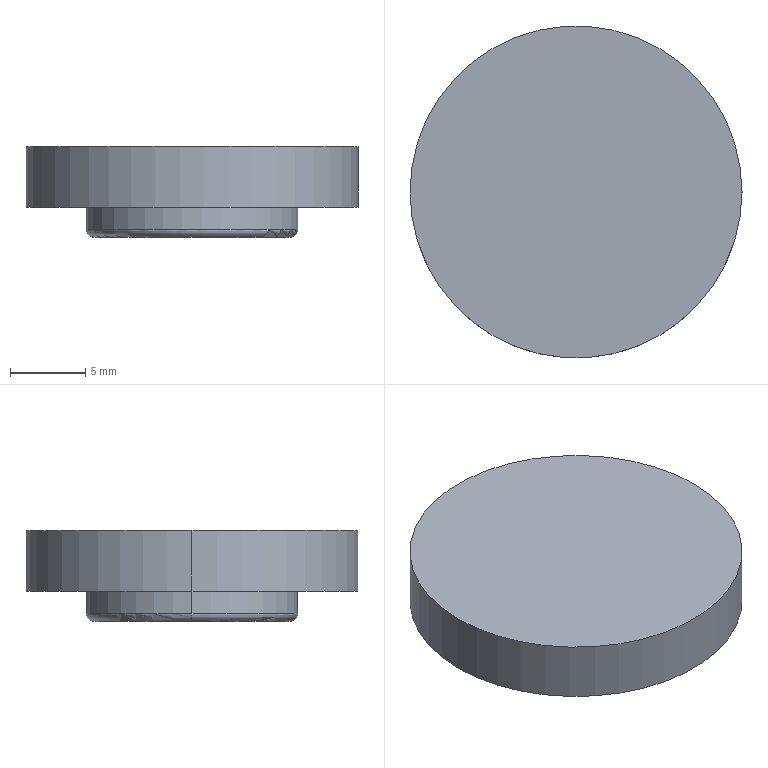Part | 1 solid | 9 faces | box 22 x 22 x 6 mm | volume 1826 mm3 | cylinder 4 | plane 3 | torus 2 | commonest cylinder face diameters 14 x2 22 x2
STEP:
#1=CARTESIAN_POINT('',(-6.5,0.,0.));
#2=VERTEX_POINT('',#1);
#3=CARTESIAN_POINT('',(6.5,0.,0.));
#4=VERTEX_POINT('',#3);
#5=CARTESIAN_POINT('',(0.,0.,0.));
#6=DIRECTION('',(0.,0.,-1.));
#7=DIRECTION('',(1.,0.,0.));
#8=AXIS2_PLACEMENT_3D('',#5,#6,#7);
#9=CIRCLE('',#8,6.5);
#10=EDGE_CURVE('',#2,#4,#9,.T.);
#11=ORIENTED_EDGE('',*,*,#10,.F.);
#12=CARTESIAN_POINT('',(-7.,0.,0.5));
#13=VERTEX_POINT('',#12);
#14=CARTESIAN_POINT('',(-6.5,0.,0.5));
#15=DIRECTION('',(0.,1.,0.));
#16=DIRECTION('',(-1.,0.,0.));
#17=AXIS2_PLACEMENT_3D('',#14,#15,#16);
#18=CIRCLE('',#17,0.5);
#19=EDGE_CURVE('',#2,#13,#18,.T.);
#20=ORIENTED_EDGE('',*,*,#19,.T.);
#21=CARTESIAN_POINT('',(7.,0.,0.5));
#22=VERTEX_POINT('',#21);
#23=CARTESIAN_POINT('',(0.,0.,0.5));
#24=DIRECTION('',(0.,0.,1.));
#25=DIRECTION('',(1.,0.,0.));
#26=AXIS2_PLACEMENT_3D('',#23,#24,#25);
#27=CIRCLE('',#26,7.);
#28=EDGE_CURVE('',#22,#13,#27,.T.);
#29=ORIENTED_EDGE('',*,*,#28,.F.);
#30=CARTESIAN_POINT('',(6.5,0.,0.5));
#31=DIRECTION('',(0.,-1.,0.));
#32=DIRECTION('',(0.,0.,-1.));
#33=AXIS2_PLACEMENT_3D('',#30,#31,#32);
#34=CIRCLE('',#33,0.5);
#35=EDGE_CURVE('',#4,#22,#34,.T.);
#36=ORIENTED_EDGE('',*,*,#35,.F.);
#37=EDGE_LOOP('',(#11,#20,#29,#36));
#38=FACE_OUTER_BOUND('',#37,.T.);
#39=CARTESIAN_POINT('',(0.,0.,0.5));
#40=DIRECTION('',(0.,0.,1.));
#41=DIRECTION('',(1.,0.,0.));
#42=AXIS2_PLACEMENT_3D('',#39,#40,#41);
#43=TOROIDAL_SURFACE('',#42,6.5,0.5);
#44=ADVANCED_FACE('',(#38),#43,.T.);
#45=CARTESIAN_POINT('',(11.,0.,6.));
#46=VERTEX_POINT('',#45);
#47=CARTESIAN_POINT('',(-11.,0.,6.));
#48=VERTEX_POINT('',#47);
#49=CARTESIAN_POINT('',(0.,0.,6.));
#50=DIRECTION('',(0.,0.,1.));
#51=DIRECTION('',(1.,0.,0.));
#52=AXIS2_PLACEMENT_3D('',#49,#50,#51);
#53=CIRCLE('',#52,11.);
#54=EDGE_CURVE('',#46,#48,#53,.T.);
#55=ORIENTED_EDGE('',*,*,#54,.F.);
#56=CARTESIAN_POINT('',(11.,0.,2.));
#57=VERTEX_POINT('',#56);
#58=CARTESIAN_POINT('',(11.,0.,6.));
#59=DIRECTION('',(0.,0.,-1.));
#60=VECTOR('',#59,1000.);
#61=LINE('',#58,#60);
#62=EDGE_CURVE('',#46,#57,#61,.T.);
#63=ORIENTED_EDGE('',*,*,#62,.T.);
#64=CARTESIAN_POINT('',(-11.,0.,2.));
#65=VERTEX_POINT('',#64);
#66=CARTESIAN_POINT('',(0.,0.,2.));
#67=DIRECTION('',(0.,0.,1.));
#68=DIRECTION('',(1.,0.,0.));
#69=AXIS2_PLACEMENT_3D('',#66,#67,#68);
#70=CIRCLE('',#69,11.);
#71=EDGE_CURVE('',#57,#65,#70,.T.);
#72=ORIENTED_EDGE('',*,*,#71,.T.);
#73=CARTESIAN_POINT('',(-11.,0.,6.));
#74=DIRECTION('',(0.,0.,-1.));
#75=VECTOR('',#74,1000.);
#76=LINE('',#73,#75);
#77=EDGE_CURVE('',#48,#65,#76,.T.);
#78=ORIENTED_EDGE('',*,*,#77,.F.);
#79=EDGE_LOOP('',(#55,#63,#72,#78));
#80=FACE_OUTER_BOUND('',#79,.T.);
#81=CARTESIAN_POINT('',(0.,0.,6.));
#82=DIRECTION('',(0.,0.,-1.));
#83=DIRECTION('',(-1.,0.,0.));
#84=AXIS2_PLACEMENT_3D('',#81,#82,#83);
#85=CYLINDRICAL_SURFACE('',#84,11.);
#86=ADVANCED_FACE('',(#80),#85,.T.);
#87=CARTESIAN_POINT('',(7.,0.,2.));
#88=VERTEX_POINT('',#87);
#89=CARTESIAN_POINT('',(-7.,0.,2.));
#90=VERTEX_POINT('',#89);
#91=CARTESIAN_POINT('',(0.,0.,2.));
#92=DIRECTION('',(0.,0.,1.));
#93=DIRECTION('',(1.,0.,0.));
#94=AXIS2_PLACEMENT_3D('',#91,#92,#93);
#95=CIRCLE('',#94,7.);
#96=EDGE_CURVE('',#88,#90,#95,.T.);
#97=ORIENTED_EDGE('',*,*,#96,.F.);
#98=CARTESIAN_POINT('',(7.,0.,2.));
#99=DIRECTION('',(0.,0.,-1.));
#100=VECTOR('',#99,1000.);
#101=LINE('',#98,#100);
#102=EDGE_CURVE('',#88,#22,#101,.T.);
#103=ORIENTED_EDGE('',*,*,#102,.T.);
#104=ORIENTED_EDGE('',*,*,#28,.T.);
#105=CARTESIAN_POINT('',(-7.,0.,2.));
#106=DIRECTION('',(0.,0.,-1.));
#107=VECTOR('',#106,1000.);
#108=LINE('',#105,#107);
#109=EDGE_CURVE('',#90,#13,#108,.T.);
#110=ORIENTED_EDGE('',*,*,#109,.F.);
#111=EDGE_LOOP('',(#97,#103,#104,#110));
#112=FACE_OUTER_BOUND('',#111,.T.);
#113=CARTESIAN_POINT('',(0.,0.,2.));
#114=DIRECTION('',(0.,0.,-1.));
#115=DIRECTION('',(-1.,0.,0.));
#116=AXIS2_PLACEMENT_3D('',#113,#114,#115);
#117=CYLINDRICAL_SURFACE('',#116,7.);
#118=ADVANCED_FACE('',(#112),#117,.T.);
#119=ORIENTED_EDGE('',*,*,#102,.F.);
#120=CARTESIAN_POINT('',(0.,0.,2.));
#121=DIRECTION('',(0.,0.,1.));
#122=DIRECTION('',(1.,0.,0.));
#123=AXIS2_PLACEMENT_3D('',#120,#121,#122);
#124=CIRCLE('',#123,7.);
#125=EDGE_CURVE('',#90,#88,#124,.T.);
#126=ORIENTED_EDGE('',*,*,#125,.F.);
#127=ORIENTED_EDGE('',*,*,#109,.T.);
#128=CARTESIAN_POINT('',(0.,0.,0.5));
#129=DIRECTION('',(0.,0.,1.));
#130=DIRECTION('',(1.,0.,0.));
#131=AXIS2_PLACEMENT_3D('',#128,#129,#130);
#132=CIRCLE('',#131,7.);
#133=EDGE_CURVE('',#13,#22,#132,.T.);
#134=ORIENTED_EDGE('',*,*,#133,.T.);
#135=EDGE_LOOP('',(#119,#126,#127,#134));
#136=FACE_OUTER_BOUND('',#135,.T.);
#137=CARTESIAN_POINT('',(0.,0.,2.));
#138=DIRECTION('',(0.,0.,-1.));
#139=DIRECTION('',(-1.,0.,0.));
#140=AXIS2_PLACEMENT_3D('',#137,#138,#139);
#141=CYLINDRICAL_SURFACE('',#140,7.);
#142=ADVANCED_FACE('',(#136),#141,.T.);
#143=CARTESIAN_POINT('',(0.,0.,0.));
#144=DIRECTION('',(0.,0.,-1.));
#145=DIRECTION('',(1.,0.,0.));
#146=AXIS2_PLACEMENT_3D('',#143,#144,#145);
#147=CIRCLE('',#146,6.5);
#148=EDGE_CURVE('',#4,#2,#147,.T.);
#149=ORIENTED_EDGE('',*,*,#148,.T.);
#150=ORIENTED_EDGE('',*,*,#10,.T.);
#151=EDGE_LOOP('',(#149,#150));
#152=FACE_OUTER_BOUND('',#151,.T.);
#153=CARTESIAN_POINT('',(0.,0.,0.));
#154=DIRECTION('',(0.,0.,1.));
#155=DIRECTION('',(1.,0.,0.));
#156=AXIS2_PLACEMENT_3D('',#153,#154,#155);
#157=PLANE('',#156);
#158=ADVANCED_FACE('',(#152),#157,.F.);
#159=ORIENTED_EDGE('',*,*,#62,.F.);
#160=CARTESIAN_POINT('',(0.,0.,6.));
#161=DIRECTION('',(0.,0.,1.));
#162=DIRECTION('',(1.,0.,0.));
#163=AXIS2_PLACEMENT_3D('',#160,#161,#162);
#164=CIRCLE('',#163,11.);
#165=EDGE_CURVE('',#48,#46,#164,.T.);
#166=ORIENTED_EDGE('',*,*,#165,.F.);
#167=ORIENTED_EDGE('',*,*,#77,.T.);
#168=CARTESIAN_POINT('',(0.,0.,2.));
#169=DIRECTION('',(0.,0.,1.));
#170=DIRECTION('',(1.,0.,0.));
#171=AXIS2_PLACEMENT_3D('',#168,#169,#170);
#172=CIRCLE('',#171,11.);
#173=EDGE_CURVE('',#65,#57,#172,.T.);
#174=ORIENTED_EDGE('',*,*,#173,.T.);
#175=EDGE_LOOP('',(#159,#166,#167,#174));
#176=FACE_OUTER_BOUND('',#175,.T.);
#177=CARTESIAN_POINT('',(0.,0.,6.));
#178=DIRECTION('',(0.,0.,-1.));
#179=DIRECTION('',(-1.,0.,0.));
#180=AXIS2_PLACEMENT_3D('',#177,#178,#179);
#181=CYLINDRICAL_SURFACE('',#180,11.);
#182=ADVANCED_FACE('',(#176),#181,.T.);
#183=ORIENTED_EDGE('',*,*,#165,.T.);
#184=ORIENTED_EDGE('',*,*,#54,.T.);
#185=EDGE_LOOP('',(#183,#184));
#186=FACE_OUTER_BOUND('',#185,.T.);
#187=CARTESIAN_POINT('',(0.,0.,6.));
#188=DIRECTION('',(0.,0.,1.));
#189=DIRECTION('',(1.,0.,0.));
#190=AXIS2_PLACEMENT_3D('',#187,#188,#189);
#191=PLANE('',#190);
#192=ADVANCED_FACE('',(#186),#191,.T.);
#193=ORIENTED_EDGE('',*,*,#173,.F.);
#194=ORIENTED_EDGE('',*,*,#71,.F.);
#195=EDGE_LOOP('',(#193,#194));
#196=FACE_OUTER_BOUND('',#195,.T.);
#197=ORIENTED_EDGE('',*,*,#125,.T.);
#198=ORIENTED_EDGE('',*,*,#96,.T.);
#199=EDGE_LOOP('',(#197,#198));
#200=FACE_BOUND('',#199,.T.);
#201=CARTESIAN_POINT('',(0.,0.,2.));
#202=DIRECTION('',(0.,0.,1.));
#203=DIRECTION('',(1.,0.,0.));
#204=AXIS2_PLACEMENT_3D('',#201,#202,#203);
#205=PLANE('',#204);
#206=ADVANCED_FACE('',(#196,#200),#205,.F.);
#207=ORIENTED_EDGE('',*,*,#19,.F.);
#208=ORIENTED_EDGE('',*,*,#148,.F.);
#209=ORIENTED_EDGE('',*,*,#35,.T.);
#210=ORIENTED_EDGE('',*,*,#133,.F.);
#211=EDGE_LOOP('',(#207,#208,#209,#210));
#212=FACE_OUTER_BOUND('',#211,.T.);
#213=CARTESIAN_POINT('',(0.,0.,0.5));
#214=DIRECTION('',(0.,0.,1.));
#215=DIRECTION('',(1.,0.,0.));
#216=AXIS2_PLACEMENT_3D('',#213,#214,#215);
#217=TOROIDAL_SURFACE('',#216,6.5,0.5);
#218=ADVANCED_FACE('',(#212),#217,.T.);
#219=CLOSED_SHELL('',(#44,#86,#118,#142,#158,#182,#192,#206,#218));
#220=MANIFOLD_SOLID_BREP('',#219);
#221=CARTESIAN_POINT('',(0.,0.,0.));
#222=DIRECTION('',(0.,0.,1.));
#223=DIRECTION('',(1.,0.,0.));
#224=AXIS2_PLACEMENT_3D('',#221,#222,#223);
#225=(LENGTH_UNIT()NAMED_UNIT(*)SI_UNIT(.MILLI.,.METRE.));
#226=UNCERTAINTY_MEASURE_WITH_UNIT(LENGTH_MEASURE(0.00001),#225,'','');
#227=(NAMED_UNIT(*)PLANE_ANGLE_UNIT()SI_UNIT($,.RADIAN.));
#228=(NAMED_UNIT(*)SI_UNIT($,.STERADIAN.)SOLID_ANGLE_UNIT());
#229=(GEOMETRIC_REPRESENTATION_CONTEXT(3)GLOBAL_UNCERTAINTY_ASSIGNED_CONTEXT((#226))GLOBAL_UNIT_ASSIGNED_CONTEXT((#225,#227,#228))REPRESENTATION_CONTEXT('',''));
#230=ADVANCED_BREP_SHAPE_REPRESENTATION('',(#220,#224),#229);